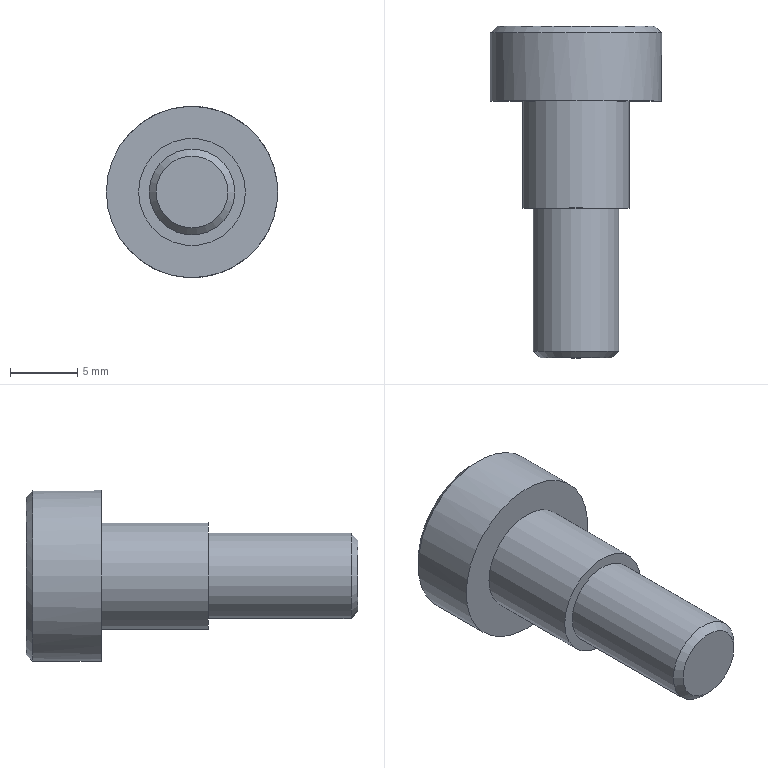Part | NX | features shoulder bolts MS51576(94035A302) 2 | 1 solid | 16 faces | box 12.7 x 24.606 x 12.7 mm | volume 1398 mm3 | plane 11 | cylinder 3 | cone 2 | commonest cylinder face diameters 6.35 x1 7.938 x1 12.7 x1
STEP:
#1=CARTESIAN_POINT('',(5.842,5.556,0.));
#2=VERTEX_POINT('',#1);
#3=CARTESIAN_POINT('',(0.,5.556,0.));
#4=DIRECTION('',(0.,-1.,0.));
#5=DIRECTION('',(1.,0.,0.));
#6=AXIS2_PLACEMENT_3D('',#3,#4,#5);
#7=CIRCLE('',#6,5.842);
#8=EDGE_CURVE('',#2,#2,#7,.F.);
#9=ORIENTED_EDGE('',*,*,#8,.T.);
#10=EDGE_LOOP('',(#9));
#11=FACE_BOUND('',#10,.T.);
#12=CARTESIAN_POINT('',(0.,5.556,-2.291));
#13=VERTEX_POINT('',#12);
#14=CARTESIAN_POINT('',(-1.984,5.556,-1.146));
#15=VERTEX_POINT('',#14);
#16=CARTESIAN_POINT('',(0.,5.556,-2.291));
#17=DIRECTION('',(-0.866,0.,0.5));
#18=VECTOR('',#17,1000.);
#19=LINE('',#16,#18);
#20=EDGE_CURVE('',#13,#15,#19,.T.);
#21=ORIENTED_EDGE('',*,*,#20,.F.);
#22=CARTESIAN_POINT('',(1.984,5.556,-1.146));
#23=VERTEX_POINT('',#22);
#24=CARTESIAN_POINT('',(1.984,5.556,-1.146));
#25=DIRECTION('',(-0.866,0.,-0.5));
#26=VECTOR('',#25,1000.);
#27=LINE('',#24,#26);
#28=EDGE_CURVE('',#23,#13,#27,.T.);
#29=ORIENTED_EDGE('',*,*,#28,.F.);
#30=CARTESIAN_POINT('',(1.984,5.556,1.146));
#31=VERTEX_POINT('',#30);
#32=CARTESIAN_POINT('',(1.984,5.556,1.146));
#33=DIRECTION('',(0.,0.,-1.));
#34=VECTOR('',#33,1000.);
#35=LINE('',#32,#34);
#36=EDGE_CURVE('',#31,#23,#35,.T.);
#37=ORIENTED_EDGE('',*,*,#36,.F.);
#38=CARTESIAN_POINT('',(0.,5.556,2.291));
#39=VERTEX_POINT('',#38);
#40=CARTESIAN_POINT('',(0.,5.556,2.291));
#41=DIRECTION('',(0.866,0.,-0.5));
#42=VECTOR('',#41,1000.);
#43=LINE('',#40,#42);
#44=EDGE_CURVE('',#39,#31,#43,.T.);
#45=ORIENTED_EDGE('',*,*,#44,.F.);
#46=CARTESIAN_POINT('',(-1.984,5.556,1.146));
#47=VERTEX_POINT('',#46);
#48=CARTESIAN_POINT('',(-1.984,5.556,1.146));
#49=DIRECTION('',(0.866,0.,0.5));
#50=VECTOR('',#49,1000.);
#51=LINE('',#48,#50);
#52=EDGE_CURVE('',#47,#39,#51,.T.);
#53=ORIENTED_EDGE('',*,*,#52,.F.);
#54=CARTESIAN_POINT('',(-1.984,5.556,-1.146));
#55=DIRECTION('',(0.,0.,1.));
#56=VECTOR('',#55,1000.);
#57=LINE('',#54,#56);
#58=EDGE_CURVE('',#15,#47,#57,.T.);
#59=ORIENTED_EDGE('',*,*,#58,.F.);
#60=EDGE_LOOP('',(#21,#29,#37,#45,#53,#59));
#61=FACE_BOUND('',#60,.T.);
#62=CARTESIAN_POINT('',(6.35,5.556,0.));
#63=DIRECTION('',(0.,-1.,0.));
#64=DIRECTION('',(1.,0.,0.));
#65=AXIS2_PLACEMENT_3D('',#62,#63,#64);
#66=PLANE('',#65);
#67=ADVANCED_FACE('',(#11,#61),#66,.F.);
#68=CARTESIAN_POINT('',(6.35,5.048,0.));
#69=VERTEX_POINT('',#68);
#70=CARTESIAN_POINT('',(0.,5.048,0.));
#71=DIRECTION('',(0.,-1.,0.));
#72=DIRECTION('',(1.,0.,0.));
#73=AXIS2_PLACEMENT_3D('',#70,#71,#72);
#74=CIRCLE('',#73,6.35);
#75=EDGE_CURVE('',#69,#69,#74,.T.);
#76=ORIENTED_EDGE('',*,*,#75,.T.);
#77=EDGE_LOOP('',(#76));
#78=FACE_BOUND('',#77,.T.);
#79=CARTESIAN_POINT('',(-6.35,0.,0.));
#80=VERTEX_POINT('',#79);
#81=CARTESIAN_POINT('',(0.,0.,0.));
#82=DIRECTION('',(0.,1.,0.));
#83=DIRECTION('',(-1.,0.,0.));
#84=AXIS2_PLACEMENT_3D('',#81,#82,#83);
#85=CIRCLE('',#84,6.35);
#86=EDGE_CURVE('',#80,#80,#85,.T.);
#87=ORIENTED_EDGE('',*,*,#86,.T.);
#88=EDGE_LOOP('',(#87));
#89=FACE_BOUND('',#88,.T.);
#90=CARTESIAN_POINT('',(0.,0.,0.));
#91=DIRECTION('',(0.,1.,0.));
#92=DIRECTION('',(-1.,0.,0.));
#93=AXIS2_PLACEMENT_3D('',#90,#91,#92);
#94=CYLINDRICAL_SURFACE('',#93,6.35);
#95=ADVANCED_FACE('',(#78,#89),#94,.T.);
#96=ORIENTED_EDGE('',*,*,#86,.F.);
#97=EDGE_LOOP('',(#96));
#98=FACE_BOUND('',#97,.T.);
#99=CARTESIAN_POINT('',(-3.969,0.,0.));
#100=VERTEX_POINT('',#99);
#101=CARTESIAN_POINT('',(0.,0.,0.));
#102=DIRECTION('',(0.,1.,0.));
#103=DIRECTION('',(-1.,0.,0.));
#104=AXIS2_PLACEMENT_3D('',#101,#102,#103);
#105=CIRCLE('',#104,3.969);
#106=EDGE_CURVE('',#100,#100,#105,.T.);
#107=ORIENTED_EDGE('',*,*,#106,.T.);
#108=EDGE_LOOP('',(#107));
#109=FACE_BOUND('',#108,.T.);
#110=CARTESIAN_POINT('',(3.969,0.,0.));
#111=DIRECTION('',(0.,1.,0.));
#112=DIRECTION('',(-1.,0.,0.));
#113=AXIS2_PLACEMENT_3D('',#110,#111,#112);
#114=PLANE('',#113);
#115=ADVANCED_FACE('',(#98,#109),#114,.F.);
#116=ORIENTED_EDGE('',*,*,#106,.F.);
#117=EDGE_LOOP('',(#116));
#118=FACE_BOUND('',#117,.T.);
#119=CARTESIAN_POINT('',(-3.969,-7.938,0.));
#120=VERTEX_POINT('',#119);
#121=CARTESIAN_POINT('',(0.,-7.938,0.));
#122=DIRECTION('',(0.,1.,0.));
#123=DIRECTION('',(-1.,0.,0.));
#124=AXIS2_PLACEMENT_3D('',#121,#122,#123);
#125=CIRCLE('',#124,3.969);
#126=EDGE_CURVE('',#120,#120,#125,.T.);
#127=ORIENTED_EDGE('',*,*,#126,.T.);
#128=EDGE_LOOP('',(#127));
#129=FACE_BOUND('',#128,.T.);
#130=CARTESIAN_POINT('',(0.,0.,0.));
#131=DIRECTION('',(0.,1.,0.));
#132=DIRECTION('',(-1.,0.,0.));
#133=AXIS2_PLACEMENT_3D('',#130,#131,#132);
#134=CYLINDRICAL_SURFACE('',#133,3.969);
#135=ADVANCED_FACE('',(#118,#129),#134,.T.);
#136=ORIENTED_EDGE('',*,*,#126,.F.);
#137=EDGE_LOOP('',(#136));
#138=FACE_BOUND('',#137,.T.);
#139=CARTESIAN_POINT('',(-3.175,-7.938,0.));
#140=VERTEX_POINT('',#139);
#141=CARTESIAN_POINT('',(0.,-7.938,0.));
#142=DIRECTION('',(0.,1.,0.));
#143=DIRECTION('',(-1.,0.,0.));
#144=AXIS2_PLACEMENT_3D('',#141,#142,#143);
#145=CIRCLE('',#144,3.175);
#146=EDGE_CURVE('',#140,#140,#145,.T.);
#147=ORIENTED_EDGE('',*,*,#146,.T.);
#148=EDGE_LOOP('',(#147));
#149=FACE_BOUND('',#148,.T.);
#150=CARTESIAN_POINT('',(3.175,-7.938,0.));
#151=DIRECTION('',(0.,1.,0.));
#152=DIRECTION('',(-1.,0.,0.));
#153=AXIS2_PLACEMENT_3D('',#150,#151,#152);
#154=PLANE('',#153);
#155=ADVANCED_FACE('',(#138,#149),#154,.F.);
#156=CARTESIAN_POINT('',(-3.175,-18.542,0.));
#157=VERTEX_POINT('',#156);
#158=CARTESIAN_POINT('',(0.,-18.542,0.));
#159=DIRECTION('',(0.,1.,0.));
#160=DIRECTION('',(-1.,0.,0.));
#161=AXIS2_PLACEMENT_3D('',#158,#159,#160);
#162=CIRCLE('',#161,3.175);
#163=EDGE_CURVE('',#157,#157,#162,.T.);
#164=ORIENTED_EDGE('',*,*,#163,.T.);
#165=EDGE_LOOP('',(#164));
#166=FACE_BOUND('',#165,.T.);
#167=ORIENTED_EDGE('',*,*,#146,.F.);
#168=EDGE_LOOP('',(#167));
#169=FACE_BOUND('',#168,.T.);
#170=CARTESIAN_POINT('',(0.,0.,0.));
#171=DIRECTION('',(0.,1.,0.));
#172=DIRECTION('',(-1.,0.,0.));
#173=AXIS2_PLACEMENT_3D('',#170,#171,#172);
#174=CYLINDRICAL_SURFACE('',#173,3.175);
#175=ADVANCED_FACE('',(#166,#169),#174,.T.);
#176=CARTESIAN_POINT('',(-2.667,-19.05,0.));
#177=VERTEX_POINT('',#176);
#178=CARTESIAN_POINT('',(0.,-19.05,0.));
#179=DIRECTION('',(0.,1.,0.));
#180=DIRECTION('',(-1.,0.,0.));
#181=AXIS2_PLACEMENT_3D('',#178,#179,#180);
#182=CIRCLE('',#181,2.667);
#183=EDGE_CURVE('',#177,#177,#182,.F.);
#184=ORIENTED_EDGE('',*,*,#183,.T.);
#185=EDGE_LOOP('',(#184));
#186=FACE_BOUND('',#185,.T.);
#187=CARTESIAN_POINT('',(0.,-19.05,0.));
#188=DIRECTION('',(0.,1.,0.));
#189=DIRECTION('',(-1.,0.,0.));
#190=AXIS2_PLACEMENT_3D('',#187,#188,#189);
#191=PLANE('',#190);
#192=ADVANCED_FACE('',(#186),#191,.F.);
#193=ORIENTED_EDGE('',*,*,#28,.T.);
#194=CARTESIAN_POINT('',(0.,2.381,-2.291));
#195=VERTEX_POINT('',#194);
#196=CARTESIAN_POINT('',(0.,2.381,-2.291));
#197=DIRECTION('',(0.,1.,0.));
#198=VECTOR('',#197,1000.);
#199=LINE('',#196,#198);
#200=EDGE_CURVE('',#195,#13,#199,.T.);
#201=ORIENTED_EDGE('',*,*,#200,.F.);
#202=CARTESIAN_POINT('',(1.984,2.381,-1.146));
#203=VERTEX_POINT('',#202);
#204=CARTESIAN_POINT('',(1.984,2.381,-1.146));
#205=DIRECTION('',(-0.866,0.,-0.5));
#206=VECTOR('',#205,1000.);
#207=LINE('',#204,#206);
#208=EDGE_CURVE('',#203,#195,#207,.T.);
#209=ORIENTED_EDGE('',*,*,#208,.F.);
#210=CARTESIAN_POINT('',(1.984,2.381,-1.146));
#211=DIRECTION('',(0.,1.,0.));
#212=VECTOR('',#211,1000.);
#213=LINE('',#210,#212);
#214=EDGE_CURVE('',#203,#23,#213,.T.);
#215=ORIENTED_EDGE('',*,*,#214,.T.);
#216=EDGE_LOOP('',(#193,#201,#209,#215));
#217=FACE_BOUND('',#216,.T.);
#218=CARTESIAN_POINT('',(1.984,2.381,-1.146));
#219=DIRECTION('',(0.5,0.,-0.866));
#220=DIRECTION('',(-0.866,0.,-0.5));
#221=AXIS2_PLACEMENT_3D('',#218,#219,#220);
#222=PLANE('',#221);
#223=ADVANCED_FACE('',(#217),#222,.F.);
#224=ORIENTED_EDGE('',*,*,#36,.T.);
#225=ORIENTED_EDGE('',*,*,#214,.F.);
#226=CARTESIAN_POINT('',(1.984,2.381,1.146));
#227=VERTEX_POINT('',#226);
#228=CARTESIAN_POINT('',(1.984,2.381,1.146));
#229=DIRECTION('',(0.,0.,-1.));
#230=VECTOR('',#229,1000.);
#231=LINE('',#228,#230);
#232=EDGE_CURVE('',#227,#203,#231,.T.);
#233=ORIENTED_EDGE('',*,*,#232,.F.);
#234=CARTESIAN_POINT('',(1.984,2.381,1.146));
#235=DIRECTION('',(0.,1.,0.));
#236=VECTOR('',#235,1000.);
#237=LINE('',#234,#236);
#238=EDGE_CURVE('',#227,#31,#237,.T.);
#239=ORIENTED_EDGE('',*,*,#238,.T.);
#240=EDGE_LOOP('',(#224,#225,#233,#239));
#241=FACE_BOUND('',#240,.T.);
#242=CARTESIAN_POINT('',(1.984,2.381,1.146));
#243=DIRECTION('',(1.,0.,0.));
#244=DIRECTION('',(0.,1.,0.));
#245=AXIS2_PLACEMENT_3D('',#242,#243,#244);
#246=PLANE('',#245);
#247=ADVANCED_FACE('',(#241),#246,.F.);
#248=ORIENTED_EDGE('',*,*,#44,.T.);
#249=ORIENTED_EDGE('',*,*,#238,.F.);
#250=CARTESIAN_POINT('',(0.,2.381,2.291));
#251=VERTEX_POINT('',#250);
#252=CARTESIAN_POINT('',(0.,2.381,2.291));
#253=DIRECTION('',(0.866,0.,-0.5));
#254=VECTOR('',#253,1000.);
#255=LINE('',#252,#254);
#256=EDGE_CURVE('',#251,#227,#255,.T.);
#257=ORIENTED_EDGE('',*,*,#256,.F.);
#258=CARTESIAN_POINT('',(0.,2.381,2.291));
#259=DIRECTION('',(0.,1.,0.));
#260=VECTOR('',#259,1000.);
#261=LINE('',#258,#260);
#262=EDGE_CURVE('',#251,#39,#261,.T.);
#263=ORIENTED_EDGE('',*,*,#262,.T.);
#264=EDGE_LOOP('',(#248,#249,#257,#263));
#265=FACE_BOUND('',#264,.T.);
#266=CARTESIAN_POINT('',(0.,2.381,2.291));
#267=DIRECTION('',(0.5,0.,0.866));
#268=DIRECTION('',(0.866,0.,-0.5));
#269=AXIS2_PLACEMENT_3D('',#266,#267,#268);
#270=PLANE('',#269);
#271=ADVANCED_FACE('',(#265),#270,.F.);
#272=ORIENTED_EDGE('',*,*,#52,.T.);
#273=ORIENTED_EDGE('',*,*,#262,.F.);
#274=CARTESIAN_POINT('',(-1.984,2.381,1.146));
#275=VERTEX_POINT('',#274);
#276=CARTESIAN_POINT('',(-1.984,2.381,1.146));
#277=DIRECTION('',(0.866,0.,0.5));
#278=VECTOR('',#277,1000.);
#279=LINE('',#276,#278);
#280=EDGE_CURVE('',#275,#251,#279,.T.);
#281=ORIENTED_EDGE('',*,*,#280,.F.);
#282=CARTESIAN_POINT('',(-1.984,2.381,1.146));
#283=DIRECTION('',(0.,1.,0.));
#284=VECTOR('',#283,1000.);
#285=LINE('',#282,#284);
#286=EDGE_CURVE('',#275,#47,#285,.T.);
#287=ORIENTED_EDGE('',*,*,#286,.T.);
#288=EDGE_LOOP('',(#272,#273,#281,#287));
#289=FACE_BOUND('',#288,.T.);
#290=CARTESIAN_POINT('',(-1.984,2.381,1.146));
#291=DIRECTION('',(-0.5,0.,0.866));
#292=DIRECTION('',(0.866,0.,0.5));
#293=AXIS2_PLACEMENT_3D('',#290,#291,#292);
#294=PLANE('',#293);
#295=ADVANCED_FACE('',(#289),#294,.F.);
#296=ORIENTED_EDGE('',*,*,#58,.T.);
#297=ORIENTED_EDGE('',*,*,#286,.F.);
#298=CARTESIAN_POINT('',(-1.984,2.381,-1.146));
#299=VERTEX_POINT('',#298);
#300=CARTESIAN_POINT('',(-1.984,2.381,-1.146));
#301=DIRECTION('',(0.,0.,1.));
#302=VECTOR('',#301,1000.);
#303=LINE('',#300,#302);
#304=EDGE_CURVE('',#299,#275,#303,.T.);
#305=ORIENTED_EDGE('',*,*,#304,.F.);
#306=CARTESIAN_POINT('',(-1.984,2.381,-1.146));
#307=DIRECTION('',(0.,1.,0.));
#308=VECTOR('',#307,1000.);
#309=LINE('',#306,#308);
#310=EDGE_CURVE('',#299,#15,#309,.T.);
#311=ORIENTED_EDGE('',*,*,#310,.T.);
#312=EDGE_LOOP('',(#296,#297,#305,#311));
#313=FACE_BOUND('',#312,.T.);
#314=CARTESIAN_POINT('',(-1.984,2.381,-1.146));
#315=DIRECTION('',(-1.,0.,0.));
#316=DIRECTION('',(0.,-1.,0.));
#317=AXIS2_PLACEMENT_3D('',#314,#315,#316);
#318=PLANE('',#317);
#319=ADVANCED_FACE('',(#313),#318,.F.);
#320=ORIENTED_EDGE('',*,*,#20,.T.);
#321=ORIENTED_EDGE('',*,*,#310,.F.);
#322=CARTESIAN_POINT('',(0.,2.381,-2.291));
#323=DIRECTION('',(-0.866,0.,0.5));
#324=VECTOR('',#323,1000.);
#325=LINE('',#322,#324);
#326=EDGE_CURVE('',#195,#299,#325,.T.);
#327=ORIENTED_EDGE('',*,*,#326,.F.);
#328=ORIENTED_EDGE('',*,*,#200,.T.);
#329=EDGE_LOOP('',(#320,#321,#327,#328));
#330=FACE_BOUND('',#329,.T.);
#331=CARTESIAN_POINT('',(0.,2.381,-2.291));
#332=DIRECTION('',(-0.5,0.,-0.866));
#333=DIRECTION('',(-0.866,0.,0.5));
#334=AXIS2_PLACEMENT_3D('',#331,#332,#333);
#335=PLANE('',#334);
#336=ADVANCED_FACE('',(#330),#335,.F.);
#337=ORIENTED_EDGE('',*,*,#208,.T.);
#338=ORIENTED_EDGE('',*,*,#326,.T.);
#339=ORIENTED_EDGE('',*,*,#304,.T.);
#340=ORIENTED_EDGE('',*,*,#280,.T.);
#341=ORIENTED_EDGE('',*,*,#256,.T.);
#342=ORIENTED_EDGE('',*,*,#232,.T.);
#343=EDGE_LOOP('',(#337,#338,#339,#340,#341,#342));
#344=FACE_BOUND('',#343,.T.);
#345=CARTESIAN_POINT('',(-1.984,2.381,-3.437));
#346=DIRECTION('',(0.,1.,0.));
#347=DIRECTION('',(0.,0.,1.));
#348=AXIS2_PLACEMENT_3D('',#345,#346,#347);
#349=PLANE('',#348);
#350=ADVANCED_FACE('',(#344),#349,.T.);
#351=ORIENTED_EDGE('',*,*,#75,.F.);
#352=EDGE_LOOP('',(#351));
#353=FACE_BOUND('',#352,.T.);
#354=ORIENTED_EDGE('',*,*,#8,.F.);
#355=EDGE_LOOP('',(#354));
#356=FACE_BOUND('',#355,.T.);
#357=CARTESIAN_POINT('',(0.,5.556,0.));
#358=DIRECTION('',(0.,-1.,0.));
#359=DIRECTION('',(1.,0.,0.));
#360=AXIS2_PLACEMENT_3D('',#357,#358,#359);
#361=CONICAL_SURFACE('',#360,5.842,0.7854);
#362=ADVANCED_FACE('',(#353,#356),#361,.T.);
#363=ORIENTED_EDGE('',*,*,#183,.F.);
#364=EDGE_LOOP('',(#363));
#365=FACE_BOUND('',#364,.T.);
#366=ORIENTED_EDGE('',*,*,#163,.F.);
#367=EDGE_LOOP('',(#366));
#368=FACE_BOUND('',#367,.T.);
#369=CARTESIAN_POINT('',(0.,-18.542,0.));
#370=DIRECTION('',(0.,1.,0.));
#371=DIRECTION('',(-1.,0.,0.));
#372=AXIS2_PLACEMENT_3D('',#369,#370,#371);
#373=CONICAL_SURFACE('',#372,3.175,0.7854);
#374=ADVANCED_FACE('',(#365,#368),#373,.T.);
#375=CLOSED_SHELL('',(#67,#95,#115,#135,#155,#175,#192,#223,#247,#271,#295,#319,#336,#350,#362,#374));
#376=MANIFOLD_SOLID_BREP('',#375);
#377=(LENGTH_UNIT()NAMED_UNIT(*)SI_UNIT(.MILLI.,.METRE.));
#378=UNCERTAINTY_MEASURE_WITH_UNIT(LENGTH_MEASURE(0.00001),#377,'','');
#379=(NAMED_UNIT(*)PLANE_ANGLE_UNIT()SI_UNIT($,.RADIAN.));
#380=(NAMED_UNIT(*)SI_UNIT($,.STERADIAN.)SOLID_ANGLE_UNIT());
#381=(GEOMETRIC_REPRESENTATION_CONTEXT(3)GLOBAL_UNCERTAINTY_ASSIGNED_CONTEXT((#378))GLOBAL_UNIT_ASSIGNED_CONTEXT((#377,#379,#380))REPRESENTATION_CONTEXT('',''));
#382=ADVANCED_BREP_SHAPE_REPRESENTATION('',(#376),#381);